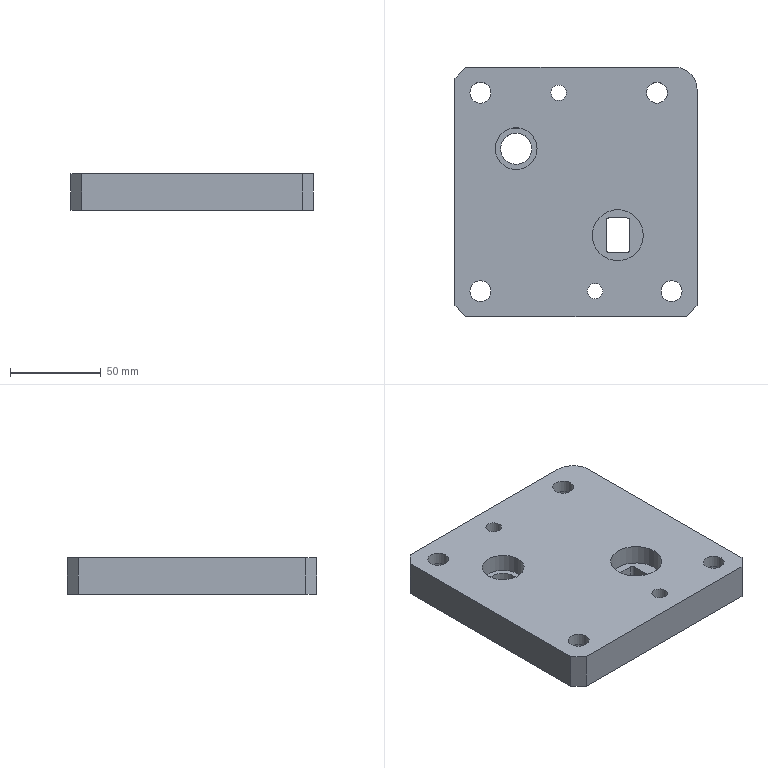Part | STEP file | lll_id3146_x_t | 1 solid | 37 faces | box 133 x 137 x 20 mm | volume 328863 mm3 | plane 19 | cylinder 18 | commonest cylinder face diameters 3 x4 11.509 x4 18.007 x4 8.506 x2 17.1 x1 23 x1
STEP:
#1=CARTESIAN_POINT('',(426.374,-378.25,2.5));
#2=VERTEX_POINT('',#1);
#3=CARTESIAN_POINT('',(417.37,-378.25,2.5));
#4=DIRECTION('',(0.,0.,1.));
#5=DIRECTION('',(1.,0.,0.));
#6=AXIS2_PLACEMENT_3D('',#3,#4,#5);
#7=CIRCLE('',#6,9.004);
#8=EDGE_CURVE('',#2,#2,#7,.T.);
#9=ORIENTED_EDGE('',*,*,#8,.T.);
#10=EDGE_LOOP('',(#9));
#11=FACE_BOUND('',#10,.T.);
#12=CARTESIAN_POINT('',(531.374,-378.25,2.5));
#13=VERTEX_POINT('',#12);
#14=CARTESIAN_POINT('',(522.37,-378.25,2.5));
#15=DIRECTION('',(0.,0.,1.));
#16=DIRECTION('',(1.,0.,0.));
#17=AXIS2_PLACEMENT_3D('',#14,#15,#16);
#18=CIRCLE('',#17,9.004);
#19=EDGE_CURVE('',#13,#13,#18,.T.);
#20=ORIENTED_EDGE('',*,*,#19,.T.);
#21=EDGE_LOOP('',(#20));
#22=FACE_BOUND('',#21,.T.);
#23=CARTESIAN_POINT('',(464.623,-269.25,2.5));
#24=VERTEX_POINT('',#23);
#25=CARTESIAN_POINT('',(460.37,-269.25,2.5));
#26=DIRECTION('',(0.,0.,1.));
#27=DIRECTION('',(1.,0.,0.));
#28=AXIS2_PLACEMENT_3D('',#25,#26,#27);
#29=CIRCLE('',#28,4.253);
#30=EDGE_CURVE('',#24,#24,#29,.T.);
#31=ORIENTED_EDGE('',*,*,#30,.T.);
#32=EDGE_LOOP('',(#31));
#33=FACE_BOUND('',#32,.T.);
#34=CARTESIAN_POINT('',(524.37,-255.25,2.5));
#35=VERTEX_POINT('',#34);
#36=CARTESIAN_POINT('',(409.37,-255.25,2.5));
#37=VERTEX_POINT('',#36);
#38=CARTESIAN_POINT('',(466.37,-255.25,2.5));
#39=DIRECTION('',(-1.,0.,0.));
#40=VECTOR('',#39,1.);
#41=LINE('',#38,#40);
#42=EDGE_CURVE('',#35,#37,#41,.T.);
#43=ORIENTED_EDGE('',*,*,#42,.F.);
#44=CARTESIAN_POINT('',(536.37,-267.25,2.5));
#45=VERTEX_POINT('',#44);
#46=CARTESIAN_POINT('',(524.37,-267.25,2.5));
#47=DIRECTION('',(0.,0.,-1.));
#48=DIRECTION('',(-1.,0.,0.));
#49=AXIS2_PLACEMENT_3D('',#46,#47,#48);
#50=CIRCLE('',#49,12.);
#51=EDGE_CURVE('',#35,#45,#50,.T.);
#52=ORIENTED_EDGE('',*,*,#51,.T.);
#53=CARTESIAN_POINT('',(536.37,-386.25,2.5));
#54=VERTEX_POINT('',#53);
#55=CARTESIAN_POINT('',(536.37,-325.25,2.5));
#56=DIRECTION('',(0.,1.,0.));
#57=VECTOR('',#56,1.);
#58=LINE('',#55,#57);
#59=EDGE_CURVE('',#54,#45,#58,.T.);
#60=ORIENTED_EDGE('',*,*,#59,.F.);
#61=CARTESIAN_POINT('',(530.37,-392.25,2.5));
#62=VERTEX_POINT('',#61);
#63=CARTESIAN_POINT('',(531.87,-390.75,2.5));
#64=DIRECTION('',(-0.7071,-0.7071,0.));
#65=VECTOR('',#64,1.);
#66=LINE('',#63,#65);
#67=EDGE_CURVE('',#54,#62,#66,.T.);
#68=ORIENTED_EDGE('',*,*,#67,.T.);
#69=CARTESIAN_POINT('',(409.37,-392.25,2.5));
#70=VERTEX_POINT('',#69);
#71=CARTESIAN_POINT('',(466.37,-392.25,2.5));
#72=DIRECTION('',(1.,0.,0.));
#73=VECTOR('',#72,1.);
#74=LINE('',#71,#73);
#75=EDGE_CURVE('',#70,#62,#74,.T.);
#76=ORIENTED_EDGE('',*,*,#75,.F.);
#77=CARTESIAN_POINT('',(403.37,-386.25,2.5));
#78=VERTEX_POINT('',#77);
#79=CARTESIAN_POINT('',(404.37,-387.25,2.5));
#80=DIRECTION('',(-0.7071,0.7071,0.));
#81=VECTOR('',#80,1.);
#82=LINE('',#79,#81);
#83=EDGE_CURVE('',#70,#78,#82,.T.);
#84=ORIENTED_EDGE('',*,*,#83,.T.);
#85=CARTESIAN_POINT('',(403.37,-261.25,2.5));
#86=VERTEX_POINT('',#85);
#87=CARTESIAN_POINT('',(403.37,-325.25,2.5));
#88=DIRECTION('',(0.,-1.,0.));
#89=VECTOR('',#88,1.);
#90=LINE('',#87,#89);
#91=EDGE_CURVE('',#86,#78,#90,.T.);
#92=ORIENTED_EDGE('',*,*,#91,.F.);
#93=CARTESIAN_POINT('',(402.87,-261.75,2.5));
#94=DIRECTION('',(0.7071,0.7071,0.));
#95=VECTOR('',#94,1.);
#96=LINE('',#93,#95);
#97=EDGE_CURVE('',#86,#37,#96,.T.);
#98=ORIENTED_EDGE('',*,*,#97,.T.);
#99=EDGE_LOOP('',(#43,#52,#60,#68,#76,#84,#92,#98));
#100=FACE_BOUND('',#99,.T.);
#101=CARTESIAN_POINT('',(497.87,-357.,2.5));
#102=VERTEX_POINT('',#101);
#103=CARTESIAN_POINT('',(487.87,-357.,2.5));
#104=VERTEX_POINT('',#103);
#105=CARTESIAN_POINT('',(466.37,-357.,2.5));
#106=DIRECTION('',(-1.,0.,0.));
#107=VECTOR('',#106,1.);
#108=LINE('',#105,#107);
#109=EDGE_CURVE('',#102,#104,#108,.T.);
#110=ORIENTED_EDGE('',*,*,#109,.F.);
#111=CARTESIAN_POINT('',(499.37,-355.5,2.5));
#112=VERTEX_POINT('',#111);
#113=CARTESIAN_POINT('',(497.87,-355.5,2.5));
#114=DIRECTION('',(0.,0.,-1.));
#115=DIRECTION('',(-1.,0.,0.));
#116=AXIS2_PLACEMENT_3D('',#113,#114,#115);
#117=CIRCLE('',#116,1.5);
#118=EDGE_CURVE('',#112,#102,#117,.T.);
#119=ORIENTED_EDGE('',*,*,#118,.F.);
#120=CARTESIAN_POINT('',(499.37,-339.5,2.5));
#121=VERTEX_POINT('',#120);
#122=CARTESIAN_POINT('',(499.37,-325.25,2.5));
#123=DIRECTION('',(0.,-1.,0.));
#124=VECTOR('',#123,1.);
#125=LINE('',#122,#124);
#126=EDGE_CURVE('',#121,#112,#125,.T.);
#127=ORIENTED_EDGE('',*,*,#126,.F.);
#128=CARTESIAN_POINT('',(497.87,-338.,2.5));
#129=VERTEX_POINT('',#128);
#130=CARTESIAN_POINT('',(497.87,-339.5,2.5));
#131=DIRECTION('',(0.,0.,-1.));
#132=DIRECTION('',(-1.,0.,0.));
#133=AXIS2_PLACEMENT_3D('',#130,#131,#132);
#134=CIRCLE('',#133,1.5);
#135=EDGE_CURVE('',#129,#121,#134,.T.);
#136=ORIENTED_EDGE('',*,*,#135,.F.);
#137=CARTESIAN_POINT('',(487.87,-338.,2.5));
#138=VERTEX_POINT('',#137);
#139=CARTESIAN_POINT('',(466.37,-338.,2.5));
#140=DIRECTION('',(1.,0.,0.));
#141=VECTOR('',#140,1.);
#142=LINE('',#139,#141);
#143=EDGE_CURVE('',#138,#129,#142,.T.);
#144=ORIENTED_EDGE('',*,*,#143,.F.);
#145=CARTESIAN_POINT('',(486.37,-339.5,2.5));
#146=VERTEX_POINT('',#145);
#147=CARTESIAN_POINT('',(487.87,-339.5,2.5));
#148=DIRECTION('',(0.,0.,-1.));
#149=DIRECTION('',(-1.,0.,0.));
#150=AXIS2_PLACEMENT_3D('',#147,#148,#149);
#151=CIRCLE('',#150,1.5);
#152=EDGE_CURVE('',#146,#138,#151,.T.);
#153=ORIENTED_EDGE('',*,*,#152,.F.);
#154=CARTESIAN_POINT('',(486.37,-355.5,2.5));
#155=VERTEX_POINT('',#154);
#156=CARTESIAN_POINT('',(486.37,-325.25,2.5));
#157=DIRECTION('',(0.,1.,0.));
#158=VECTOR('',#157,1.);
#159=LINE('',#156,#158);
#160=EDGE_CURVE('',#155,#146,#159,.T.);
#161=ORIENTED_EDGE('',*,*,#160,.F.);
#162=CARTESIAN_POINT('',(487.87,-355.5,2.5));
#163=DIRECTION('',(0.,0.,-1.));
#164=DIRECTION('',(-1.,0.,0.));
#165=AXIS2_PLACEMENT_3D('',#162,#163,#164);
#166=CIRCLE('',#165,1.5);
#167=EDGE_CURVE('',#104,#155,#166,.T.);
#168=ORIENTED_EDGE('',*,*,#167,.F.);
#169=EDGE_LOOP('',(#110,#119,#127,#136,#144,#153,#161,#168));
#170=FACE_BOUND('',#169,.T.);
#171=CARTESIAN_POINT('',(428.45,-300.,2.5));
#172=VERTEX_POINT('',#171);
#173=CARTESIAN_POINT('',(437.,-300.,2.5));
#174=DIRECTION('',(0.,0.,1.));
#175=DIRECTION('',(-1.,0.,0.));
#176=AXIS2_PLACEMENT_3D('',#173,#174,#175);
#177=CIRCLE('',#176,8.55);
#178=EDGE_CURVE('',#172,#172,#177,.T.);
#179=ORIENTED_EDGE('',*,*,#178,.T.);
#180=EDGE_LOOP('',(#179));
#181=FACE_BOUND('',#180,.T.);
#182=CARTESIAN_POINT('',(484.623,-378.25,2.5));
#183=VERTEX_POINT('',#182);
#184=CARTESIAN_POINT('',(480.37,-378.25,2.5));
#185=DIRECTION('',(0.,0.,1.));
#186=DIRECTION('',(1.,0.,0.));
#187=AXIS2_PLACEMENT_3D('',#184,#185,#186);
#188=CIRCLE('',#187,4.253);
#189=EDGE_CURVE('',#183,#183,#188,.T.);
#190=ORIENTED_EDGE('',*,*,#189,.T.);
#191=EDGE_LOOP('',(#190));
#192=FACE_BOUND('',#191,.T.);
#193=CARTESIAN_POINT('',(523.374,-269.25,2.5));
#194=VERTEX_POINT('',#193);
#195=CARTESIAN_POINT('',(514.37,-269.25,2.5));
#196=DIRECTION('',(0.,0.,1.));
#197=DIRECTION('',(1.,0.,0.));
#198=AXIS2_PLACEMENT_3D('',#195,#196,#197);
#199=CIRCLE('',#198,9.004);
#200=EDGE_CURVE('',#194,#194,#199,.T.);
#201=ORIENTED_EDGE('',*,*,#200,.T.);
#202=EDGE_LOOP('',(#201));
#203=FACE_BOUND('',#202,.T.);
#204=CARTESIAN_POINT('',(426.374,-269.25,2.5));
#205=VERTEX_POINT('',#204);
#206=CARTESIAN_POINT('',(417.37,-269.25,2.5));
#207=DIRECTION('',(0.,0.,1.));
#208=DIRECTION('',(1.,0.,0.));
#209=AXIS2_PLACEMENT_3D('',#206,#207,#208);
#210=CIRCLE('',#209,9.004);
#211=EDGE_CURVE('',#205,#205,#210,.T.);
#212=ORIENTED_EDGE('',*,*,#211,.T.);
#213=EDGE_LOOP('',(#212));
#214=FACE_BOUND('',#213,.T.);
#215=CARTESIAN_POINT('',(466.37,-325.25,2.5));
#216=DIRECTION('',(0.,0.,-1.));
#217=DIRECTION('',(0.,-1.,0.));
#218=AXIS2_PLACEMENT_3D('',#215,#216,#217);
#219=PLANE('',#218);
#220=ADVANCED_FACE('',(#11,#22,#33,#100,#170,#181,#192,#203,#214),#219,.T.);
#221=CARTESIAN_POINT('',(497.87,-357.,11.5));
#222=VERTEX_POINT('',#221);
#223=CARTESIAN_POINT('',(487.87,-357.,11.5));
#224=VERTEX_POINT('',#223);
#225=CARTESIAN_POINT('',(487.87,-357.,11.5));
#226=DIRECTION('',(-1.,0.,0.));
#227=VECTOR('',#226,1.);
#228=LINE('',#225,#227);
#229=EDGE_CURVE('',#222,#224,#228,.T.);
#230=ORIENTED_EDGE('',*,*,#229,.F.);
#231=CARTESIAN_POINT('',(497.87,-357.,-7.5));
#232=DIRECTION('',(0.,0.,-1.));
#233=VECTOR('',#232,1.);
#234=LINE('',#231,#233);
#235=EDGE_CURVE('',#222,#102,#234,.T.);
#236=ORIENTED_EDGE('',*,*,#235,.T.);
#237=ORIENTED_EDGE('',*,*,#109,.T.);
#238=CARTESIAN_POINT('',(487.87,-357.,-7.5));
#239=DIRECTION('',(0.,0.,-1.));
#240=VECTOR('',#239,1.);
#241=LINE('',#238,#240);
#242=EDGE_CURVE('',#224,#104,#241,.T.);
#243=ORIENTED_EDGE('',*,*,#242,.F.);
#244=EDGE_LOOP('',(#230,#236,#237,#243));
#245=FACE_OUTER_BOUND('',#244,.T.);
#246=CARTESIAN_POINT('',(487.87,-357.,-7.5));
#247=DIRECTION('',(0.,-1.,0.));
#248=DIRECTION('',(1.,0.,0.));
#249=AXIS2_PLACEMENT_3D('',#246,#247,#248);
#250=PLANE('',#249);
#251=ADVANCED_FACE('',(#245),#250,.F.);
#252=CARTESIAN_POINT('',(486.37,-355.5,11.5));
#253=VERTEX_POINT('',#252);
#254=CARTESIAN_POINT('',(487.87,-355.5,11.5));
#255=DIRECTION('',(0.,0.,-1.));
#256=DIRECTION('',(1.,0.,0.));
#257=AXIS2_PLACEMENT_3D('',#254,#255,#256);
#258=CIRCLE('',#257,1.5);
#259=EDGE_CURVE('',#224,#253,#258,.T.);
#260=ORIENTED_EDGE('',*,*,#259,.F.);
#261=ORIENTED_EDGE('',*,*,#242,.T.);
#262=ORIENTED_EDGE('',*,*,#167,.T.);
#263=CARTESIAN_POINT('',(486.37,-355.5,-7.5));
#264=DIRECTION('',(0.,0.,-1.));
#265=VECTOR('',#264,1.);
#266=LINE('',#263,#265);
#267=EDGE_CURVE('',#253,#155,#266,.T.);
#268=ORIENTED_EDGE('',*,*,#267,.F.);
#269=EDGE_LOOP('',(#260,#261,#262,#268));
#270=FACE_OUTER_BOUND('',#269,.T.);
#271=CARTESIAN_POINT('',(487.87,-355.5,-7.5));
#272=DIRECTION('',(0.,0.,-1.));
#273=DIRECTION('',(1.,0.,0.));
#274=AXIS2_PLACEMENT_3D('',#271,#272,#273);
#275=CYLINDRICAL_SURFACE('',#274,1.5);
#276=ADVANCED_FACE('',(#270),#275,.F.);
#277=CARTESIAN_POINT('',(486.37,-339.5,11.5));
#278=VERTEX_POINT('',#277);
#279=CARTESIAN_POINT('',(487.87,-338.,11.5));
#280=VERTEX_POINT('',#279);
#281=CARTESIAN_POINT('',(487.87,-339.5,11.5));
#282=DIRECTION('',(0.,0.,-1.));
#283=DIRECTION('',(1.,0.,0.));
#284=AXIS2_PLACEMENT_3D('',#281,#282,#283);
#285=CIRCLE('',#284,1.5);
#286=EDGE_CURVE('',#278,#280,#285,.T.);
#287=ORIENTED_EDGE('',*,*,#286,.F.);
#288=CARTESIAN_POINT('',(486.37,-339.5,-7.5));
#289=DIRECTION('',(0.,0.,-1.));
#290=VECTOR('',#289,1.);
#291=LINE('',#288,#290);
#292=EDGE_CURVE('',#278,#146,#291,.T.);
#293=ORIENTED_EDGE('',*,*,#292,.T.);
#294=ORIENTED_EDGE('',*,*,#152,.T.);
#295=CARTESIAN_POINT('',(487.87,-338.,-7.5));
#296=DIRECTION('',(0.,0.,-1.));
#297=VECTOR('',#296,1.);
#298=LINE('',#295,#297);
#299=EDGE_CURVE('',#280,#138,#298,.T.);
#300=ORIENTED_EDGE('',*,*,#299,.F.);
#301=EDGE_LOOP('',(#287,#293,#294,#300));
#302=FACE_OUTER_BOUND('',#301,.T.);
#303=CARTESIAN_POINT('',(487.87,-339.5,-7.5));
#304=DIRECTION('',(0.,0.,-1.));
#305=DIRECTION('',(1.,0.,0.));
#306=AXIS2_PLACEMENT_3D('',#303,#304,#305);
#307=CYLINDRICAL_SURFACE('',#306,1.5);
#308=ADVANCED_FACE('',(#302),#307,.F.);
#309=CARTESIAN_POINT('',(497.87,-338.,11.5));
#310=VERTEX_POINT('',#309);
#311=CARTESIAN_POINT('',(497.87,-338.,11.5));
#312=DIRECTION('',(1.,0.,0.));
#313=VECTOR('',#312,1.);
#314=LINE('',#311,#313);
#315=EDGE_CURVE('',#280,#310,#314,.T.);
#316=ORIENTED_EDGE('',*,*,#315,.F.);
#317=ORIENTED_EDGE('',*,*,#299,.T.);
#318=ORIENTED_EDGE('',*,*,#143,.T.);
#319=CARTESIAN_POINT('',(497.87,-338.,-7.5));
#320=DIRECTION('',(0.,0.,-1.));
#321=VECTOR('',#320,1.);
#322=LINE('',#319,#321);
#323=EDGE_CURVE('',#310,#129,#322,.T.);
#324=ORIENTED_EDGE('',*,*,#323,.F.);
#325=EDGE_LOOP('',(#316,#317,#318,#324));
#326=FACE_OUTER_BOUND('',#325,.T.);
#327=CARTESIAN_POINT('',(497.87,-338.,-7.5));
#328=DIRECTION('',(0.,1.,0.));
#329=DIRECTION('',(-1.,0.,0.));
#330=AXIS2_PLACEMENT_3D('',#327,#328,#329);
#331=PLANE('',#330);
#332=ADVANCED_FACE('',(#326),#331,.F.);
#333=CARTESIAN_POINT('',(499.37,-339.5,11.5));
#334=VERTEX_POINT('',#333);
#335=CARTESIAN_POINT('',(497.87,-339.5,11.5));
#336=DIRECTION('',(0.,0.,-1.));
#337=DIRECTION('',(1.,0.,0.));
#338=AXIS2_PLACEMENT_3D('',#335,#336,#337);
#339=CIRCLE('',#338,1.5);
#340=EDGE_CURVE('',#310,#334,#339,.T.);
#341=ORIENTED_EDGE('',*,*,#340,.F.);
#342=ORIENTED_EDGE('',*,*,#323,.T.);
#343=ORIENTED_EDGE('',*,*,#135,.T.);
#344=CARTESIAN_POINT('',(499.37,-339.5,-7.5));
#345=DIRECTION('',(0.,0.,-1.));
#346=VECTOR('',#345,1.);
#347=LINE('',#344,#346);
#348=EDGE_CURVE('',#334,#121,#347,.T.);
#349=ORIENTED_EDGE('',*,*,#348,.F.);
#350=EDGE_LOOP('',(#341,#342,#343,#349));
#351=FACE_OUTER_BOUND('',#350,.T.);
#352=CARTESIAN_POINT('',(497.87,-339.5,-7.5));
#353=DIRECTION('',(0.,0.,-1.));
#354=DIRECTION('',(1.,0.,0.));
#355=AXIS2_PLACEMENT_3D('',#352,#353,#354);
#356=CYLINDRICAL_SURFACE('',#355,1.5);
#357=ADVANCED_FACE('',(#351),#356,.F.);
#358=CARTESIAN_POINT('',(499.37,-355.5,11.5));
#359=VERTEX_POINT('',#358);
#360=CARTESIAN_POINT('',(497.87,-355.5,11.5));
#361=DIRECTION('',(0.,0.,-1.));
#362=DIRECTION('',(1.,0.,0.));
#363=AXIS2_PLACEMENT_3D('',#360,#361,#362);
#364=CIRCLE('',#363,1.5);
#365=EDGE_CURVE('',#359,#222,#364,.T.);
#366=ORIENTED_EDGE('',*,*,#365,.F.);
#367=CARTESIAN_POINT('',(499.37,-355.5,-7.5));
#368=DIRECTION('',(0.,0.,-1.));
#369=VECTOR('',#368,1.);
#370=LINE('',#367,#369);
#371=EDGE_CURVE('',#359,#112,#370,.T.);
#372=ORIENTED_EDGE('',*,*,#371,.T.);
#373=ORIENTED_EDGE('',*,*,#118,.T.);
#374=ORIENTED_EDGE('',*,*,#235,.F.);
#375=EDGE_LOOP('',(#366,#372,#373,#374));
#376=FACE_OUTER_BOUND('',#375,.T.);
#377=CARTESIAN_POINT('',(497.87,-355.5,-7.5));
#378=DIRECTION('',(0.,0.,-1.));
#379=DIRECTION('',(1.,0.,0.));
#380=AXIS2_PLACEMENT_3D('',#377,#378,#379);
#381=CYLINDRICAL_SURFACE('',#380,1.5);
#382=ADVANCED_FACE('',(#376),#381,.F.);
#383=CARTESIAN_POINT('',(486.37,-339.5,11.5));
#384=DIRECTION('',(0.,1.,0.));
#385=VECTOR('',#384,1.);
#386=LINE('',#383,#385);
#387=EDGE_CURVE('',#253,#278,#386,.T.);
#388=ORIENTED_EDGE('',*,*,#387,.F.);
#389=ORIENTED_EDGE('',*,*,#267,.T.);
#390=ORIENTED_EDGE('',*,*,#160,.T.);
#391=ORIENTED_EDGE('',*,*,#292,.F.);
#392=EDGE_LOOP('',(#388,#389,#390,#391));
#393=FACE_OUTER_BOUND('',#392,.T.);
#394=CARTESIAN_POINT('',(486.37,-339.5,-7.5));
#395=DIRECTION('',(-1.,0.,0.));
#396=DIRECTION('',(0.,-1.,0.));
#397=AXIS2_PLACEMENT_3D('',#394,#395,#396);
#398=PLANE('',#397);
#399=ADVANCED_FACE('',(#393),#398,.F.);
#400=CARTESIAN_POINT('',(499.37,-355.5,11.5));
#401=DIRECTION('',(0.,-1.,0.));
#402=VECTOR('',#401,1.);
#403=LINE('',#400,#402);
#404=EDGE_CURVE('',#334,#359,#403,.T.);
#405=ORIENTED_EDGE('',*,*,#404,.F.);
#406=ORIENTED_EDGE('',*,*,#348,.T.);
#407=ORIENTED_EDGE('',*,*,#126,.T.);
#408=ORIENTED_EDGE('',*,*,#371,.F.);
#409=EDGE_LOOP('',(#405,#406,#407,#408));
#410=FACE_OUTER_BOUND('',#409,.T.);
#411=CARTESIAN_POINT('',(499.37,-355.5,-7.5));
#412=DIRECTION('',(1.,0.,0.));
#413=DIRECTION('',(0.,1.,0.));
#414=AXIS2_PLACEMENT_3D('',#411,#412,#413);
#415=PLANE('',#414);
#416=ADVANCED_FACE('',(#410),#415,.F.);
#417=CARTESIAN_POINT('',(423.125,-269.25,22.5));
#418=VERTEX_POINT('',#417);
#419=CARTESIAN_POINT('',(417.37,-269.25,22.5));
#420=DIRECTION('',(0.,0.,1.));
#421=DIRECTION('',(1.,0.,0.));
#422=AXIS2_PLACEMENT_3D('',#419,#420,#421);
#423=CIRCLE('',#422,5.755);
#424=EDGE_CURVE('',#418,#418,#423,.T.);
#425=ORIENTED_EDGE('',*,*,#424,.F.);
#426=EDGE_LOOP('',(#425));
#427=FACE_BOUND('',#426,.T.);
#428=CARTESIAN_POINT('',(423.125,-378.25,22.5));
#429=VERTEX_POINT('',#428);
#430=CARTESIAN_POINT('',(417.37,-378.25,22.5));
#431=DIRECTION('',(0.,0.,1.));
#432=DIRECTION('',(1.,0.,0.));
#433=AXIS2_PLACEMENT_3D('',#430,#431,#432);
#434=CIRCLE('',#433,5.755);
#435=EDGE_CURVE('',#429,#429,#434,.T.);
#436=ORIENTED_EDGE('',*,*,#435,.F.);
#437=EDGE_LOOP('',(#436));
#438=FACE_BOUND('',#437,.T.);
#439=CARTESIAN_POINT('',(520.125,-269.25,22.5));
#440=VERTEX_POINT('',#439);
#441=CARTESIAN_POINT('',(514.37,-269.25,22.5));
#442=DIRECTION('',(0.,0.,1.));
#443=DIRECTION('',(1.,0.,0.));
#444=AXIS2_PLACEMENT_3D('',#441,#442,#443);
#445=CIRCLE('',#444,5.755);
#446=EDGE_CURVE('',#440,#440,#445,.T.);
#447=ORIENTED_EDGE('',*,*,#446,.F.);
#448=EDGE_LOOP('',(#447));
#449=FACE_BOUND('',#448,.T.);
#450=CARTESIAN_POINT('',(528.125,-378.25,22.5));
#451=VERTEX_POINT('',#450);
#452=CARTESIAN_POINT('',(522.37,-378.25,22.5));
#453=DIRECTION('',(0.,0.,1.));
#454=DIRECTION('',(1.,0.,0.));
#455=AXIS2_PLACEMENT_3D('',#452,#453,#454);
#456=CIRCLE('',#455,5.755);
#457=EDGE_CURVE('',#451,#451,#456,.T.);
#458=ORIENTED_EDGE('',*,*,#457,.F.);
#459=EDGE_LOOP('',(#458));
#460=FACE_BOUND('',#459,.T.);
#461=CARTESIAN_POINT('',(484.623,-378.25,22.5));
#462=VERTEX_POINT('',#461);
#463=CARTESIAN_POINT('',(480.37,-378.25,22.5));
#464=DIRECTION('',(0.,0.,1.));
#465=DIRECTION('',(1.,0.,0.));
#466=AXIS2_PLACEMENT_3D('',#463,#464,#465);
#467=CIRCLE('',#466,4.253);
#468=EDGE_CURVE('',#462,#462,#467,.T.);
#469=ORIENTED_EDGE('',*,*,#468,.F.);
#470=EDGE_LOOP('',(#469));
#471=FACE_BOUND('',#470,.T.);
#472=CARTESIAN_POINT('',(464.623,-269.25,22.5));
#473=VERTEX_POINT('',#472);
#474=CARTESIAN_POINT('',(460.37,-269.25,22.5));
#475=DIRECTION('',(0.,0.,1.));
#476=DIRECTION('',(1.,0.,0.));
#477=AXIS2_PLACEMENT_3D('',#474,#475,#476);
#478=CIRCLE('',#477,4.253);
#479=EDGE_CURVE('',#473,#473,#478,.T.);
#480=ORIENTED_EDGE('',*,*,#479,.F.);
#481=EDGE_LOOP('',(#480));
#482=FACE_BOUND('',#481,.T.);
#483=CARTESIAN_POINT('',(506.87,-347.5,22.5));
#484=VERTEX_POINT('',#483);
#485=CARTESIAN_POINT('',(492.87,-347.5,22.5));
#486=DIRECTION('',(0.,0.,1.));
#487=DIRECTION('',(1.,0.,0.));
#488=AXIS2_PLACEMENT_3D('',#485,#486,#487);
#489=CIRCLE('',#488,14.);
#490=EDGE_CURVE('',#484,#484,#489,.T.);
#491=ORIENTED_EDGE('',*,*,#490,.F.);
#492=EDGE_LOOP('',(#491));
#493=FACE_BOUND('',#492,.T.);
#494=CARTESIAN_POINT('',(536.37,-267.25,22.5));
#495=VERTEX_POINT('',#494);
#496=CARTESIAN_POINT('',(536.37,-386.25,22.5));
#497=VERTEX_POINT('',#496);
#498=CARTESIAN_POINT('',(536.37,-325.25,22.5));
#499=DIRECTION('',(0.,-1.,0.));
#500=VECTOR('',#499,1.);
#501=LINE('',#498,#500);
#502=EDGE_CURVE('',#495,#497,#501,.T.);
#503=ORIENTED_EDGE('',*,*,#502,.F.);
#504=CARTESIAN_POINT('',(524.37,-255.25,22.5));
#505=VERTEX_POINT('',#504);
#506=CARTESIAN_POINT('',(524.37,-267.25,22.5));
#507=DIRECTION('',(0.,0.,1.));
#508=DIRECTION('',(1.,0.,0.));
#509=AXIS2_PLACEMENT_3D('',#506,#507,#508);
#510=CIRCLE('',#509,12.);
#511=EDGE_CURVE('',#495,#505,#510,.T.);
#512=ORIENTED_EDGE('',*,*,#511,.T.);
#513=CARTESIAN_POINT('',(409.37,-255.25,22.5));
#514=VERTEX_POINT('',#513);
#515=CARTESIAN_POINT('',(466.37,-255.25,22.5));
#516=DIRECTION('',(1.,0.,0.));
#517=VECTOR('',#516,1.);
#518=LINE('',#515,#517);
#519=EDGE_CURVE('',#514,#505,#518,.T.);
#520=ORIENTED_EDGE('',*,*,#519,.F.);
#521=CARTESIAN_POINT('',(403.37,-261.25,22.5));
#522=VERTEX_POINT('',#521);
#523=CARTESIAN_POINT('',(402.87,-261.75,22.5));
#524=DIRECTION('',(-0.7071,-0.7071,0.));
#525=VECTOR('',#524,1.);
#526=LINE('',#523,#525);
#527=EDGE_CURVE('',#514,#522,#526,.T.);
#528=ORIENTED_EDGE('',*,*,#527,.T.);
#529=CARTESIAN_POINT('',(403.37,-386.25,22.5));
#530=VERTEX_POINT('',#529);
#531=CARTESIAN_POINT('',(403.37,-325.25,22.5));
#532=DIRECTION('',(0.,1.,0.));
#533=VECTOR('',#532,1.);
#534=LINE('',#531,#533);
#535=EDGE_CURVE('',#530,#522,#534,.T.);
#536=ORIENTED_EDGE('',*,*,#535,.F.);
#537=CARTESIAN_POINT('',(409.37,-392.25,22.5));
#538=VERTEX_POINT('',#537);
#539=CARTESIAN_POINT('',(404.37,-387.25,22.5));
#540=DIRECTION('',(0.7071,-0.7071,0.));
#541=VECTOR('',#540,1.);
#542=LINE('',#539,#541);
#543=EDGE_CURVE('',#530,#538,#542,.T.);
#544=ORIENTED_EDGE('',*,*,#543,.T.);
#545=CARTESIAN_POINT('',(530.37,-392.25,22.5));
#546=VERTEX_POINT('',#545);
#547=CARTESIAN_POINT('',(466.37,-392.25,22.5));
#548=DIRECTION('',(-1.,0.,0.));
#549=VECTOR('',#548,1.);
#550=LINE('',#547,#549);
#551=EDGE_CURVE('',#546,#538,#550,.T.);
#552=ORIENTED_EDGE('',*,*,#551,.F.);
#553=CARTESIAN_POINT('',(531.87,-390.75,22.5));
#554=DIRECTION('',(0.7071,0.7071,0.));
#555=VECTOR('',#554,1.);
#556=LINE('',#553,#555);
#557=EDGE_CURVE('',#546,#497,#556,.T.);
#558=ORIENTED_EDGE('',*,*,#557,.T.);
#559=EDGE_LOOP('',(#503,#512,#520,#528,#536,#544,#552,#558));
#560=FACE_BOUND('',#559,.T.);
#561=CARTESIAN_POINT('',(448.5,-300.,22.5));
#562=VERTEX_POINT('',#561);
#563=CARTESIAN_POINT('',(437.,-300.,22.5));
#564=DIRECTION('',(0.,0.,-1.));
#565=DIRECTION('',(1.,0.,0.));
#566=AXIS2_PLACEMENT_3D('',#563,#564,#565);
#567=CIRCLE('',#566,11.5);
#568=EDGE_CURVE('',#562,#562,#567,.T.);
#569=ORIENTED_EDGE('',*,*,#568,.T.);
#570=EDGE_LOOP('',(#569));
#571=FACE_BOUND('',#570,.T.);
#572=CARTESIAN_POINT('',(466.37,-325.25,22.5));
#573=DIRECTION('',(0.,0.,1.));
#574=DIRECTION('',(0.,1.,0.));
#575=AXIS2_PLACEMENT_3D('',#572,#573,#574);
#576=PLANE('',#575);
#577=ADVANCED_FACE('',(#427,#438,#449,#460,#471,#482,#493,#560,#571),#576,.T.);
#578=ORIENTED_EDGE('',*,*,#59,.T.);
#579=CARTESIAN_POINT('',(536.37,-267.25,2.5));
#580=DIRECTION('',(0.,0.,1.));
#581=VECTOR('',#580,1.);
#582=LINE('',#579,#581);
#583=EDGE_CURVE('',#45,#495,#582,.T.);
#584=ORIENTED_EDGE('',*,*,#583,.T.);
#585=ORIENTED_EDGE('',*,*,#502,.T.);
#586=CARTESIAN_POINT('',(536.37,-386.25,2.5));
#587=DIRECTION('',(0.,0.,-1.));
#588=VECTOR('',#587,1.);
#589=LINE('',#586,#588);
#590=EDGE_CURVE('',#497,#54,#589,.T.);
#591=ORIENTED_EDGE('',*,*,#590,.T.);
#592=EDGE_LOOP('',(#578,#584,#585,#591));
#593=FACE_OUTER_BOUND('',#592,.T.);
#594=CARTESIAN_POINT('',(536.37,-325.25,2.5));
#595=DIRECTION('',(1.,0.,0.));
#596=DIRECTION('',(0.,0.,-1.));
#597=AXIS2_PLACEMENT_3D('',#594,#595,#596);
#598=PLANE('',#597);
#599=ADVANCED_FACE('',(#593),#598,.T.);
#600=ORIENTED_EDGE('',*,*,#75,.T.);
#601=CARTESIAN_POINT('',(530.37,-392.25,2.5));
#602=DIRECTION('',(0.,0.,1.));
#603=VECTOR('',#602,1.);
#604=LINE('',#601,#603);
#605=EDGE_CURVE('',#62,#546,#604,.T.);
#606=ORIENTED_EDGE('',*,*,#605,.T.);
#607=ORIENTED_EDGE('',*,*,#551,.T.);
#608=CARTESIAN_POINT('',(409.37,-392.25,2.5));
#609=DIRECTION('',(0.,0.,-1.));
#610=VECTOR('',#609,1.);
#611=LINE('',#608,#610);
#612=EDGE_CURVE('',#538,#70,#611,.T.);
#613=ORIENTED_EDGE('',*,*,#612,.T.);
#614=EDGE_LOOP('',(#600,#606,#607,#613));
#615=FACE_OUTER_BOUND('',#614,.T.);
#616=CARTESIAN_POINT('',(466.37,-392.25,2.5));
#617=DIRECTION('',(0.,-1.,0.));
#618=DIRECTION('',(0.,0.,1.));
#619=AXIS2_PLACEMENT_3D('',#616,#617,#618);
#620=PLANE('',#619);
#621=ADVANCED_FACE('',(#615),#620,.T.);
#622=ORIENTED_EDGE('',*,*,#91,.T.);
#623=CARTESIAN_POINT('',(403.37,-386.25,2.5));
#624=DIRECTION('',(0.,0.,1.));
#625=VECTOR('',#624,1.);
#626=LINE('',#623,#625);
#627=EDGE_CURVE('',#78,#530,#626,.T.);
#628=ORIENTED_EDGE('',*,*,#627,.T.);
#629=ORIENTED_EDGE('',*,*,#535,.T.);
#630=CARTESIAN_POINT('',(403.37,-261.25,2.5));
#631=DIRECTION('',(0.,0.,-1.));
#632=VECTOR('',#631,1.);
#633=LINE('',#630,#632);
#634=EDGE_CURVE('',#522,#86,#633,.T.);
#635=ORIENTED_EDGE('',*,*,#634,.T.);
#636=EDGE_LOOP('',(#622,#628,#629,#635));
#637=FACE_OUTER_BOUND('',#636,.T.);
#638=CARTESIAN_POINT('',(403.37,-325.25,2.5));
#639=DIRECTION('',(-1.,0.,0.));
#640=DIRECTION('',(0.,0.,1.));
#641=AXIS2_PLACEMENT_3D('',#638,#639,#640);
#642=PLANE('',#641);
#643=ADVANCED_FACE('',(#637),#642,.T.);
#644=ORIENTED_EDGE('',*,*,#519,.T.);
#645=CARTESIAN_POINT('',(524.37,-255.25,2.5));
#646=DIRECTION('',(0.,0.,-1.));
#647=VECTOR('',#646,1.);
#648=LINE('',#645,#647);
#649=EDGE_CURVE('',#505,#35,#648,.T.);
#650=ORIENTED_EDGE('',*,*,#649,.T.);
#651=ORIENTED_EDGE('',*,*,#42,.T.);
#652=CARTESIAN_POINT('',(409.37,-255.25,2.5));
#653=DIRECTION('',(0.,0.,1.));
#654=VECTOR('',#653,1.);
#655=LINE('',#652,#654);
#656=EDGE_CURVE('',#37,#514,#655,.T.);
#657=ORIENTED_EDGE('',*,*,#656,.T.);
#658=EDGE_LOOP('',(#644,#650,#651,#657));
#659=FACE_OUTER_BOUND('',#658,.T.);
#660=CARTESIAN_POINT('',(466.37,-255.25,2.5));
#661=DIRECTION('',(0.,1.,0.));
#662=DIRECTION('',(0.,0.,-1.));
#663=AXIS2_PLACEMENT_3D('',#660,#661,#662);
#664=PLANE('',#663);
#665=ADVANCED_FACE('',(#659),#664,.T.);
#666=CARTESIAN_POINT('',(428.45,-300.,12.5));
#667=VERTEX_POINT('',#666);
#668=CARTESIAN_POINT('',(437.,-300.,12.5));
#669=DIRECTION('',(0.,0.,-1.));
#670=DIRECTION('',(-1.,0.,0.));
#671=AXIS2_PLACEMENT_3D('',#668,#669,#670);
#672=CIRCLE('',#671,8.55);
#673=EDGE_CURVE('',#667,#667,#672,.T.);
#674=ORIENTED_EDGE('',*,*,#673,.F.);
#675=EDGE_LOOP('',(#674));
#676=FACE_BOUND('',#675,.T.);
#677=ORIENTED_EDGE('',*,*,#178,.F.);
#678=EDGE_LOOP('',(#677));
#679=FACE_BOUND('',#678,.T.);
#680=CARTESIAN_POINT('',(437.,-300.,125.));
#681=DIRECTION('',(0.,0.,-1.));
#682=DIRECTION('',(1.,0.,0.));
#683=AXIS2_PLACEMENT_3D('',#680,#681,#682);
#684=CYLINDRICAL_SURFACE('',#683,8.55);
#685=ADVANCED_FACE('',(#676,#679),#684,.F.);
#686=CARTESIAN_POINT('',(425.5,-300.,12.5));
#687=VERTEX_POINT('',#686);
#688=CARTESIAN_POINT('',(437.,-300.,12.5));
#689=DIRECTION('',(0.,0.,1.));
#690=DIRECTION('',(-1.,0.,0.));
#691=AXIS2_PLACEMENT_3D('',#688,#689,#690);
#692=CIRCLE('',#691,11.5);
#693=EDGE_CURVE('',#687,#687,#692,.T.);
#694=ORIENTED_EDGE('',*,*,#693,.F.);
#695=EDGE_LOOP('',(#694));
#696=FACE_BOUND('',#695,.T.);
#697=ORIENTED_EDGE('',*,*,#568,.F.);
#698=EDGE_LOOP('',(#697));
#699=FACE_BOUND('',#698,.T.);
#700=CARTESIAN_POINT('',(437.,-300.,12.5));
#701=DIRECTION('',(0.,0.,1.));
#702=DIRECTION('',(1.,0.,0.));
#703=AXIS2_PLACEMENT_3D('',#700,#701,#702);
#704=CYLINDRICAL_SURFACE('',#703,11.5);
#705=ADVANCED_FACE('',(#696,#699),#704,.F.);
#706=ORIENTED_EDGE('',*,*,#673,.T.);
#707=EDGE_LOOP('',(#706));
#708=FACE_BOUND('',#707,.T.);
#709=ORIENTED_EDGE('',*,*,#693,.T.);
#710=EDGE_LOOP('',(#709));
#711=FACE_BOUND('',#710,.T.);
#712=CARTESIAN_POINT('',(437.,-300.,12.5));
#713=DIRECTION('',(0.,0.,-1.));
#714=DIRECTION('',(-1.,0.,0.));
#715=AXIS2_PLACEMENT_3D('',#712,#713,#714);
#716=PLANE('',#715);
#717=ADVANCED_FACE('',(#708,#711),#716,.F.);
#718=ORIENTED_EDGE('',*,*,#490,.T.);
#719=EDGE_LOOP('',(#718));
#720=FACE_BOUND('',#719,.T.);
#721=CARTESIAN_POINT('',(506.87,-347.5,11.5));
#722=VERTEX_POINT('',#721);
#723=CARTESIAN_POINT('',(492.87,-347.5,11.5));
#724=DIRECTION('',(0.,0.,1.));
#725=DIRECTION('',(1.,0.,0.));
#726=AXIS2_PLACEMENT_3D('',#723,#724,#725);
#727=CIRCLE('',#726,14.);
#728=EDGE_CURVE('',#722,#722,#727,.T.);
#729=ORIENTED_EDGE('',*,*,#728,.F.);
#730=EDGE_LOOP('',(#729));
#731=FACE_BOUND('',#730,.T.);
#732=CARTESIAN_POINT('',(492.87,-347.5,39.));
#733=DIRECTION('',(0.,0.,1.));
#734=DIRECTION('',(1.,0.,0.));
#735=AXIS2_PLACEMENT_3D('',#732,#733,#734);
#736=CYLINDRICAL_SURFACE('',#735,14.);
#737=ADVANCED_FACE('',(#720,#731),#736,.F.);
#738=ORIENTED_EDGE('',*,*,#728,.T.);
#739=EDGE_LOOP('',(#738));
#740=FACE_BOUND('',#739,.T.);
#741=ORIENTED_EDGE('',*,*,#259,.T.);
#742=ORIENTED_EDGE('',*,*,#387,.T.);
#743=ORIENTED_EDGE('',*,*,#286,.T.);
#744=ORIENTED_EDGE('',*,*,#315,.T.);
#745=ORIENTED_EDGE('',*,*,#340,.T.);
#746=ORIENTED_EDGE('',*,*,#404,.T.);
#747=ORIENTED_EDGE('',*,*,#365,.T.);
#748=ORIENTED_EDGE('',*,*,#229,.T.);
#749=EDGE_LOOP('',(#741,#742,#743,#744,#745,#746,#747,#748));
#750=FACE_BOUND('',#749,.T.);
#751=CARTESIAN_POINT('',(492.87,-347.5,11.5));
#752=DIRECTION('',(0.,0.,1.));
#753=DIRECTION('',(1.,0.,0.));
#754=AXIS2_PLACEMENT_3D('',#751,#752,#753);
#755=PLANE('',#754);
#756=ADVANCED_FACE('',(#740,#750),#755,.T.);
#757=ORIENTED_EDGE('',*,*,#479,.T.);
#758=EDGE_LOOP('',(#757));
#759=FACE_BOUND('',#758,.T.);
#760=ORIENTED_EDGE('',*,*,#30,.F.);
#761=EDGE_LOOP('',(#760));
#762=FACE_BOUND('',#761,.T.);
#763=CARTESIAN_POINT('',(460.37,-269.25,2.5));
#764=DIRECTION('',(0.,0.,1.));
#765=DIRECTION('',(1.,0.,0.));
#766=AXIS2_PLACEMENT_3D('',#763,#764,#765);
#767=CYLINDRICAL_SURFACE('',#766,4.253);
#768=ADVANCED_FACE('',(#759,#762),#767,.F.);
#769=ORIENTED_EDGE('',*,*,#468,.T.);
#770=EDGE_LOOP('',(#769));
#771=FACE_BOUND('',#770,.T.);
#772=ORIENTED_EDGE('',*,*,#189,.F.);
#773=EDGE_LOOP('',(#772));
#774=FACE_BOUND('',#773,.T.);
#775=CARTESIAN_POINT('',(480.37,-378.25,2.5));
#776=DIRECTION('',(0.,0.,1.));
#777=DIRECTION('',(1.,0.,0.));
#778=AXIS2_PLACEMENT_3D('',#775,#776,#777);
#779=CYLINDRICAL_SURFACE('',#778,4.253);
#780=ADVANCED_FACE('',(#771,#774),#779,.F.);
#781=ORIENTED_EDGE('',*,*,#457,.T.);
#782=EDGE_LOOP('',(#781));
#783=FACE_BOUND('',#782,.T.);
#784=CARTESIAN_POINT('',(528.125,-378.25,15.5));
#785=VERTEX_POINT('',#784);
#786=CARTESIAN_POINT('',(522.37,-378.25,15.5));
#787=DIRECTION('',(0.,0.,1.));
#788=DIRECTION('',(1.,0.,0.));
#789=AXIS2_PLACEMENT_3D('',#786,#787,#788);
#790=CIRCLE('',#789,5.755);
#791=EDGE_CURVE('',#785,#785,#790,.T.);
#792=ORIENTED_EDGE('',*,*,#791,.F.);
#793=EDGE_LOOP('',(#792));
#794=FACE_BOUND('',#793,.T.);
#795=CARTESIAN_POINT('',(522.37,-378.25,-2.5));
#796=DIRECTION('',(0.,0.,1.));
#797=DIRECTION('',(1.,0.,0.));
#798=AXIS2_PLACEMENT_3D('',#795,#796,#797);
#799=CYLINDRICAL_SURFACE('',#798,5.755);
#800=ADVANCED_FACE('',(#783,#794),#799,.F.);
#801=ORIENTED_EDGE('',*,*,#791,.T.);
#802=EDGE_LOOP('',(#801));
#803=FACE_BOUND('',#802,.T.);
#804=CARTESIAN_POINT('',(531.374,-378.25,15.5));
#805=VERTEX_POINT('',#804);
#806=CARTESIAN_POINT('',(522.37,-378.25,15.5));
#807=DIRECTION('',(0.,0.,1.));
#808=DIRECTION('',(1.,0.,0.));
#809=AXIS2_PLACEMENT_3D('',#806,#807,#808);
#810=CIRCLE('',#809,9.004);
#811=EDGE_CURVE('',#805,#805,#810,.T.);
#812=ORIENTED_EDGE('',*,*,#811,.F.);
#813=EDGE_LOOP('',(#812));
#814=FACE_BOUND('',#813,.T.);
#815=CARTESIAN_POINT('',(522.37,-378.25,15.5));
#816=DIRECTION('',(0.,0.,1.));
#817=DIRECTION('',(1.,0.,0.));
#818=AXIS2_PLACEMENT_3D('',#815,#816,#817);
#819=PLANE('',#818);
#820=ADVANCED_FACE('',(#803,#814),#819,.F.);
#821=ORIENTED_EDGE('',*,*,#811,.T.);
#822=EDGE_LOOP('',(#821));
#823=FACE_BOUND('',#822,.T.);
#824=ORIENTED_EDGE('',*,*,#19,.F.);
#825=EDGE_LOOP('',(#824));
#826=FACE_BOUND('',#825,.T.);
#827=CARTESIAN_POINT('',(522.37,-378.25,2.5));
#828=DIRECTION('',(0.,0.,1.));
#829=DIRECTION('',(1.,0.,0.));
#830=AXIS2_PLACEMENT_3D('',#827,#828,#829);
#831=CYLINDRICAL_SURFACE('',#830,9.004);
#832=ADVANCED_FACE('',(#823,#826),#831,.F.);
#833=ORIENTED_EDGE('',*,*,#446,.T.);
#834=EDGE_LOOP('',(#833));
#835=FACE_BOUND('',#834,.T.);
#836=CARTESIAN_POINT('',(520.125,-269.25,15.5));
#837=VERTEX_POINT('',#836);
#838=CARTESIAN_POINT('',(514.37,-269.25,15.5));
#839=DIRECTION('',(0.,0.,1.));
#840=DIRECTION('',(1.,0.,0.));
#841=AXIS2_PLACEMENT_3D('',#838,#839,#840);
#842=CIRCLE('',#841,5.755);
#843=EDGE_CURVE('',#837,#837,#842,.T.);
#844=ORIENTED_EDGE('',*,*,#843,.F.);
#845=EDGE_LOOP('',(#844));
#846=FACE_BOUND('',#845,.T.);
#847=CARTESIAN_POINT('',(514.37,-269.25,-2.5));
#848=DIRECTION('',(0.,0.,1.));
#849=DIRECTION('',(1.,0.,0.));
#850=AXIS2_PLACEMENT_3D('',#847,#848,#849);
#851=CYLINDRICAL_SURFACE('',#850,5.755);
#852=ADVANCED_FACE('',(#835,#846),#851,.F.);
#853=ORIENTED_EDGE('',*,*,#843,.T.);
#854=EDGE_LOOP('',(#853));
#855=FACE_BOUND('',#854,.T.);
#856=CARTESIAN_POINT('',(523.374,-269.25,15.5));
#857=VERTEX_POINT('',#856);
#858=CARTESIAN_POINT('',(514.37,-269.25,15.5));
#859=DIRECTION('',(0.,0.,1.));
#860=DIRECTION('',(1.,0.,0.));
#861=AXIS2_PLACEMENT_3D('',#858,#859,#860);
#862=CIRCLE('',#861,9.004);
#863=EDGE_CURVE('',#857,#857,#862,.T.);
#864=ORIENTED_EDGE('',*,*,#863,.F.);
#865=EDGE_LOOP('',(#864));
#866=FACE_BOUND('',#865,.T.);
#867=CARTESIAN_POINT('',(514.37,-269.25,15.5));
#868=DIRECTION('',(0.,0.,1.));
#869=DIRECTION('',(1.,0.,0.));
#870=AXIS2_PLACEMENT_3D('',#867,#868,#869);
#871=PLANE('',#870);
#872=ADVANCED_FACE('',(#855,#866),#871,.F.);
#873=ORIENTED_EDGE('',*,*,#863,.T.);
#874=EDGE_LOOP('',(#873));
#875=FACE_BOUND('',#874,.T.);
#876=ORIENTED_EDGE('',*,*,#200,.F.);
#877=EDGE_LOOP('',(#876));
#878=FACE_BOUND('',#877,.T.);
#879=CARTESIAN_POINT('',(514.37,-269.25,2.5));
#880=DIRECTION('',(0.,0.,1.));
#881=DIRECTION('',(1.,0.,0.));
#882=AXIS2_PLACEMENT_3D('',#879,#880,#881);
#883=CYLINDRICAL_SURFACE('',#882,9.004);
#884=ADVANCED_FACE('',(#875,#878),#883,.F.);
#885=ORIENTED_EDGE('',*,*,#435,.T.);
#886=EDGE_LOOP('',(#885));
#887=FACE_BOUND('',#886,.T.);
#888=CARTESIAN_POINT('',(423.125,-378.25,15.5));
#889=VERTEX_POINT('',#888);
#890=CARTESIAN_POINT('',(417.37,-378.25,15.5));
#891=DIRECTION('',(0.,0.,1.));
#892=DIRECTION('',(1.,0.,0.));
#893=AXIS2_PLACEMENT_3D('',#890,#891,#892);
#894=CIRCLE('',#893,5.755);
#895=EDGE_CURVE('',#889,#889,#894,.T.);
#896=ORIENTED_EDGE('',*,*,#895,.F.);
#897=EDGE_LOOP('',(#896));
#898=FACE_BOUND('',#897,.T.);
#899=CARTESIAN_POINT('',(417.37,-378.25,-2.5));
#900=DIRECTION('',(0.,0.,1.));
#901=DIRECTION('',(1.,0.,0.));
#902=AXIS2_PLACEMENT_3D('',#899,#900,#901);
#903=CYLINDRICAL_SURFACE('',#902,5.755);
#904=ADVANCED_FACE('',(#887,#898),#903,.F.);
#905=ORIENTED_EDGE('',*,*,#895,.T.);
#906=EDGE_LOOP('',(#905));
#907=FACE_BOUND('',#906,.T.);
#908=CARTESIAN_POINT('',(426.374,-378.25,15.5));
#909=VERTEX_POINT('',#908);
#910=CARTESIAN_POINT('',(417.37,-378.25,15.5));
#911=DIRECTION('',(0.,0.,1.));
#912=DIRECTION('',(1.,0.,0.));
#913=AXIS2_PLACEMENT_3D('',#910,#911,#912);
#914=CIRCLE('',#913,9.004);
#915=EDGE_CURVE('',#909,#909,#914,.T.);
#916=ORIENTED_EDGE('',*,*,#915,.F.);
#917=EDGE_LOOP('',(#916));
#918=FACE_BOUND('',#917,.T.);
#919=CARTESIAN_POINT('',(417.37,-378.25,15.5));
#920=DIRECTION('',(0.,0.,1.));
#921=DIRECTION('',(1.,0.,0.));
#922=AXIS2_PLACEMENT_3D('',#919,#920,#921);
#923=PLANE('',#922);
#924=ADVANCED_FACE('',(#907,#918),#923,.F.);
#925=ORIENTED_EDGE('',*,*,#915,.T.);
#926=EDGE_LOOP('',(#925));
#927=FACE_BOUND('',#926,.T.);
#928=ORIENTED_EDGE('',*,*,#8,.F.);
#929=EDGE_LOOP('',(#928));
#930=FACE_BOUND('',#929,.T.);
#931=CARTESIAN_POINT('',(417.37,-378.25,2.5));
#932=DIRECTION('',(0.,0.,1.));
#933=DIRECTION('',(1.,0.,0.));
#934=AXIS2_PLACEMENT_3D('',#931,#932,#933);
#935=CYLINDRICAL_SURFACE('',#934,9.004);
#936=ADVANCED_FACE('',(#927,#930),#935,.F.);
#937=ORIENTED_EDGE('',*,*,#424,.T.);
#938=EDGE_LOOP('',(#937));
#939=FACE_BOUND('',#938,.T.);
#940=CARTESIAN_POINT('',(423.125,-269.25,15.5));
#941=VERTEX_POINT('',#940);
#942=CARTESIAN_POINT('',(417.37,-269.25,15.5));
#943=DIRECTION('',(0.,0.,1.));
#944=DIRECTION('',(1.,0.,0.));
#945=AXIS2_PLACEMENT_3D('',#942,#943,#944);
#946=CIRCLE('',#945,5.755);
#947=EDGE_CURVE('',#941,#941,#946,.T.);
#948=ORIENTED_EDGE('',*,*,#947,.F.);
#949=EDGE_LOOP('',(#948));
#950=FACE_BOUND('',#949,.T.);
#951=CARTESIAN_POINT('',(417.37,-269.25,-2.5));
#952=DIRECTION('',(0.,0.,1.));
#953=DIRECTION('',(1.,0.,0.));
#954=AXIS2_PLACEMENT_3D('',#951,#952,#953);
#955=CYLINDRICAL_SURFACE('',#954,5.755);
#956=ADVANCED_FACE('',(#939,#950),#955,.F.);
#957=ORIENTED_EDGE('',*,*,#947,.T.);
#958=EDGE_LOOP('',(#957));
#959=FACE_BOUND('',#958,.T.);
#960=CARTESIAN_POINT('',(426.374,-269.25,15.5));
#961=VERTEX_POINT('',#960);
#962=CARTESIAN_POINT('',(417.37,-269.25,15.5));
#963=DIRECTION('',(0.,0.,1.));
#964=DIRECTION('',(1.,0.,0.));
#965=AXIS2_PLACEMENT_3D('',#962,#963,#964);
#966=CIRCLE('',#965,9.004);
#967=EDGE_CURVE('',#961,#961,#966,.T.);
#968=ORIENTED_EDGE('',*,*,#967,.F.);
#969=EDGE_LOOP('',(#968));
#970=FACE_BOUND('',#969,.T.);
#971=CARTESIAN_POINT('',(417.37,-269.25,15.5));
#972=DIRECTION('',(0.,0.,1.));
#973=DIRECTION('',(1.,0.,0.));
#974=AXIS2_PLACEMENT_3D('',#971,#972,#973);
#975=PLANE('',#974);
#976=ADVANCED_FACE('',(#959,#970),#975,.F.);
#977=ORIENTED_EDGE('',*,*,#967,.T.);
#978=EDGE_LOOP('',(#977));
#979=FACE_BOUND('',#978,.T.);
#980=ORIENTED_EDGE('',*,*,#211,.F.);
#981=EDGE_LOOP('',(#980));
#982=FACE_BOUND('',#981,.T.);
#983=CARTESIAN_POINT('',(417.37,-269.25,2.5));
#984=DIRECTION('',(0.,0.,1.));
#985=DIRECTION('',(1.,0.,0.));
#986=AXIS2_PLACEMENT_3D('',#983,#984,#985);
#987=CYLINDRICAL_SURFACE('',#986,9.004);
#988=ADVANCED_FACE('',(#979,#982),#987,.F.);
#989=ORIENTED_EDGE('',*,*,#67,.F.);
#990=ORIENTED_EDGE('',*,*,#590,.F.);
#991=ORIENTED_EDGE('',*,*,#557,.F.);
#992=ORIENTED_EDGE('',*,*,#605,.F.);
#993=EDGE_LOOP('',(#989,#990,#991,#992));
#994=FACE_OUTER_BOUND('',#993,.T.);
#995=CARTESIAN_POINT('',(530.37,-392.25,2.5));
#996=DIRECTION('',(-0.7071,0.7071,0.));
#997=DIRECTION('',(0.7071,0.7071,0.));
#998=AXIS2_PLACEMENT_3D('',#995,#996,#997);
#999=PLANE('',#998);
#1000=ADVANCED_FACE('',(#994),#999,.F.);
#1001=ORIENTED_EDGE('',*,*,#83,.F.);
#1002=ORIENTED_EDGE('',*,*,#612,.F.);
#1003=ORIENTED_EDGE('',*,*,#543,.F.);
#1004=ORIENTED_EDGE('',*,*,#627,.F.);
#1005=EDGE_LOOP('',(#1001,#1002,#1003,#1004));
#1006=FACE_OUTER_BOUND('',#1005,.T.);
#1007=CARTESIAN_POINT('',(403.37,-386.25,2.5));
#1008=DIRECTION('',(0.7071,0.7071,0.));
#1009=DIRECTION('',(0.7071,-0.7071,0.));
#1010=AXIS2_PLACEMENT_3D('',#1007,#1008,#1009);
#1011=PLANE('',#1010);
#1012=ADVANCED_FACE('',(#1006),#1011,.F.);
#1013=ORIENTED_EDGE('',*,*,#97,.F.);
#1014=ORIENTED_EDGE('',*,*,#634,.F.);
#1015=ORIENTED_EDGE('',*,*,#527,.F.);
#1016=ORIENTED_EDGE('',*,*,#656,.F.);
#1017=EDGE_LOOP('',(#1013,#1014,#1015,#1016));
#1018=FACE_OUTER_BOUND('',#1017,.T.);
#1019=CARTESIAN_POINT('',(409.37,-255.25,2.5));
#1020=DIRECTION('',(0.7071,-0.7071,0.));
#1021=DIRECTION('',(-0.7071,-0.7071,0.));
#1022=AXIS2_PLACEMENT_3D('',#1019,#1020,#1021);
#1023=PLANE('',#1022);
#1024=ADVANCED_FACE('',(#1018),#1023,.F.);
#1025=ORIENTED_EDGE('',*,*,#511,.F.);
#1026=ORIENTED_EDGE('',*,*,#583,.F.);
#1027=ORIENTED_EDGE('',*,*,#51,.F.);
#1028=ORIENTED_EDGE('',*,*,#649,.F.);
#1029=EDGE_LOOP('',(#1025,#1026,#1027,#1028));
#1030=FACE_OUTER_BOUND('',#1029,.T.);
#1031=CARTESIAN_POINT('',(524.37,-267.25,2.5));
#1032=DIRECTION('',(0.,0.,-1.));
#1033=DIRECTION('',(1.,0.,0.));
#1034=AXIS2_PLACEMENT_3D('',#1031,#1032,#1033);
#1035=CYLINDRICAL_SURFACE('',#1034,12.);
#1036=ADVANCED_FACE('',(#1030),#1035,.T.);
#1037=CLOSED_SHELL('',(#220,#251,#276,#308,#332,#357,#382,#399,#416,#577,#599,#621,#643,#665,#685,#705,#717,#737,#756,#768,#780,#800,#820,#832,#852,#872,#884,#904,#924,#936,#956,#976,#988,#1000,#1012,#1024,#1036));
#1038=MANIFOLD_SOLID_BREP('',#1037);
#1039=(LENGTH_UNIT()NAMED_UNIT(*)SI_UNIT(.MILLI.,.METRE.));
#1040=UNCERTAINTY_MEASURE_WITH_UNIT(LENGTH_MEASURE(0.00002),#1039,'','');
#1041=(NAMED_UNIT(*)PLANE_ANGLE_UNIT()SI_UNIT($,.RADIAN.));
#1042=PLANE_ANGLE_MEASURE_WITH_UNIT(PLANE_ANGLE_MEASURE(0.01745),#1041);
#1043=DIMENSIONAL_EXPONENTS(0.,0.,0.,0.,0.,0.,0.);
#1044=(CONVERSION_BASED_UNIT('DEGREE',#1042)NAMED_UNIT(#1043)PLANE_ANGLE_UNIT());
#1045=(NAMED_UNIT(*)SI_UNIT($,.STERADIAN.)SOLID_ANGLE_UNIT());
#1046=(GEOMETRIC_REPRESENTATION_CONTEXT(3)GLOBAL_UNCERTAINTY_ASSIGNED_CONTEXT((#1040))GLOBAL_UNIT_ASSIGNED_CONTEXT((#1039,#1044,#1045))REPRESENTATION_CONTEXT('',''));
#1047=ADVANCED_BREP_SHAPE_REPRESENTATION('',(#1038),#1046);